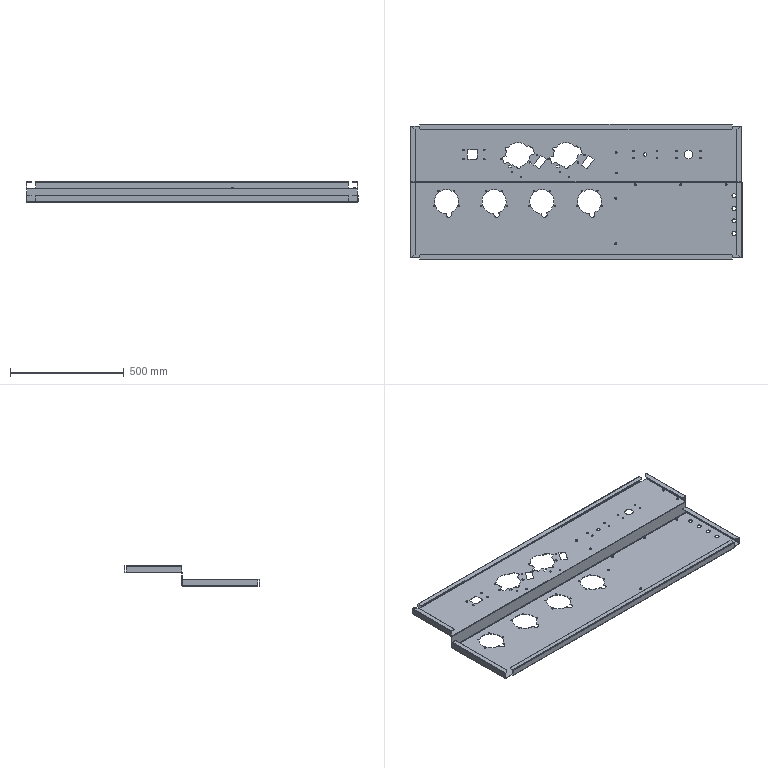Part | SolidWorks | features ICE 14, Cut 9, EdgeFlange 7, LPattern 7, Fillet 6, 3DProfileFeature 5, HoleWzd 5, Chamfer 1, FlatPattern 1, SMBaseFlange 1, SheetMetal 1 | 1 solid | 433 faces | box 1460 x 594.237 x 88.5 mm | volume 1606970 mm3 | cylinder 256 | plane 177 | commonest cylinder face diameters 2.5 x32 5 x32 6.4 x32 6 x26 106 x22 4.2 x18